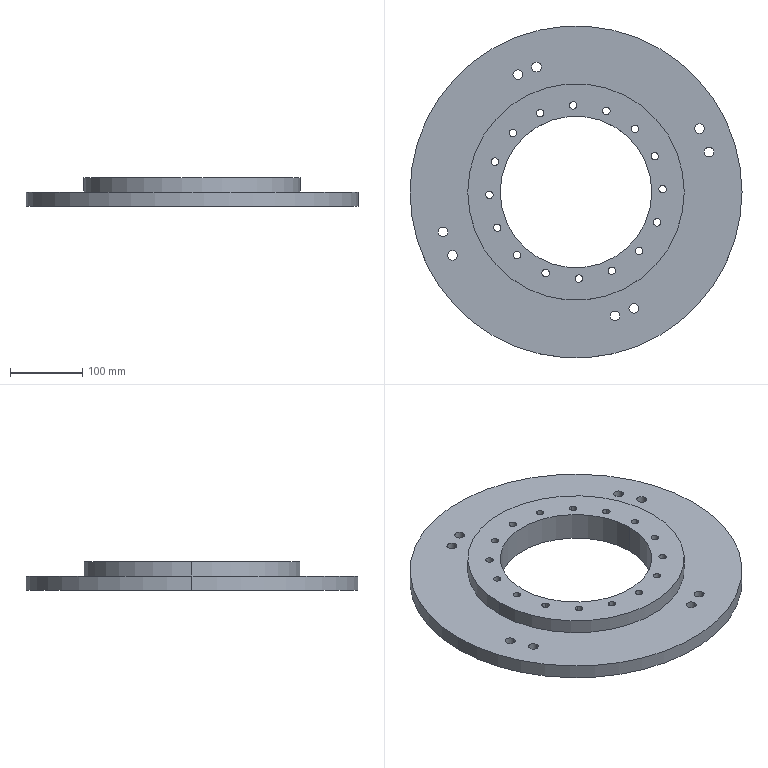Part | SolidWorks | features HoleWzd 2, ICE 2, CirPattern 1, Extrusion 1 | 1 solid | 57 faces | box 460 x 460 x 40 mm | volume 3276881 mm3 | cylinder 54 | plane 3 | commonest cylinder face diameters 10.2 x32 13.5 x16 210 x2 300 x2 460 x2